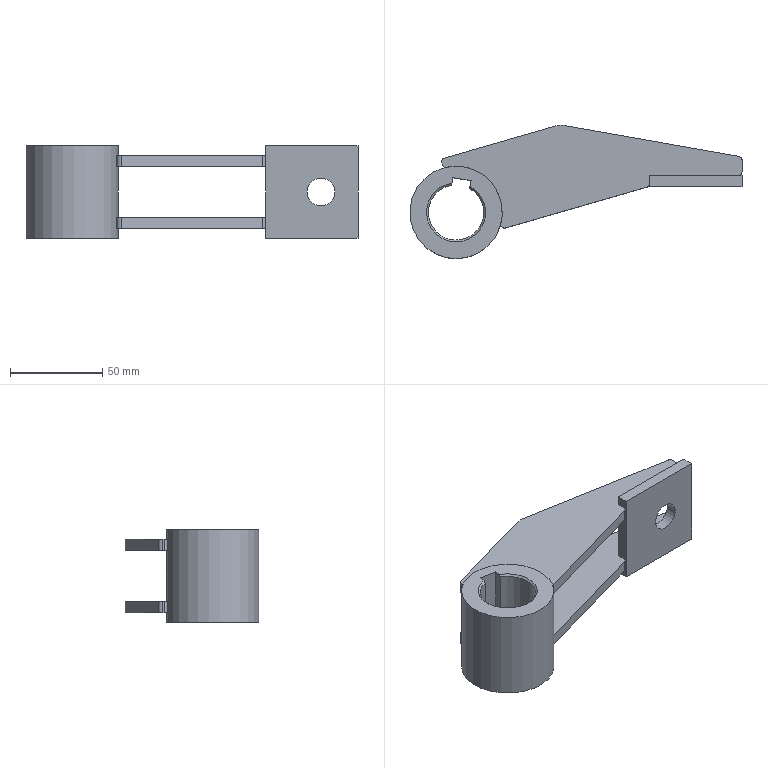Part | STEP file | HL4GZ-1.313.025 (lower steering tie-rod weldment) | 4 solids | 50 faces | box 179.65 x 72.156 x 50 mm | volume 127271 mm3 | plane 29 | cylinder 19 | cone 2 | commonest cylinder face diameters 4 x12 50 x3 20 x2 15 x1 30 x1